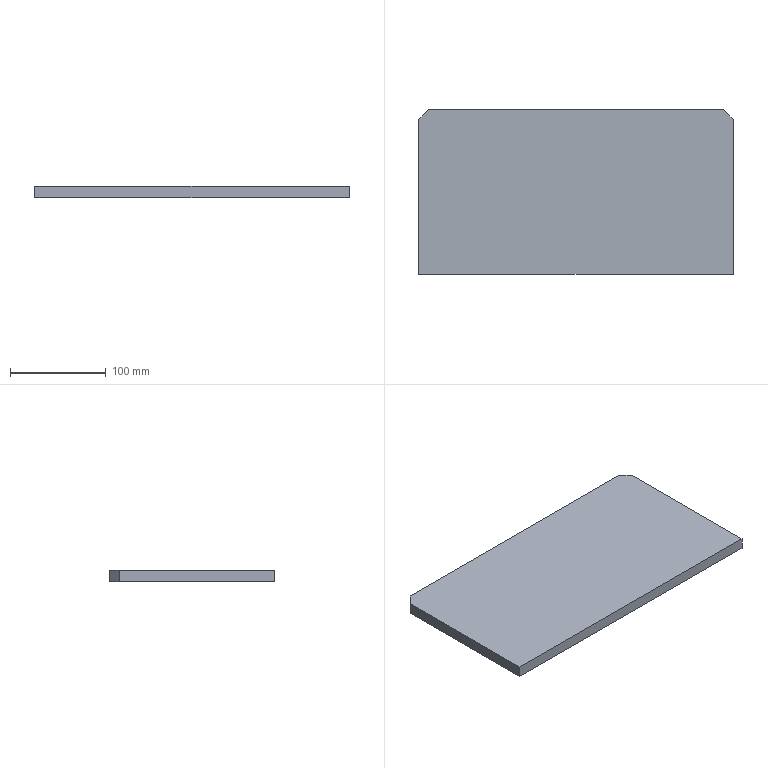Part | SolidWorks | features BaseBody 1 | 1 solid | 8 faces | box 328 x 172 x 12 mm | volume 675792 mm3 | plane 8
STEP:
#1=CARTESIAN_POINT('',(164.,-84.5,0.));
#2=VERTEX_POINT('',#1);
#3=CARTESIAN_POINT('',(164.,-84.5,12.));
#4=VERTEX_POINT('',#3);
#5=CARTESIAN_POINT('',(164.,-84.5,12.));
#6=DIRECTION('',(0.,0.,1.));
#7=VECTOR('',#6,1000.);
#8=LINE('',#5,#7);
#9=EDGE_CURVE('',#2,#4,#8,.T.);
#10=ORIENTED_EDGE('',*,*,#9,.F.);
#11=CARTESIAN_POINT('',(164.,77.5,0.));
#12=VERTEX_POINT('',#11);
#13=CARTESIAN_POINT('',(164.,77.5,0.));
#14=DIRECTION('',(0.,1.,0.));
#15=VECTOR('',#14,1000.);
#16=LINE('',#13,#15);
#17=EDGE_CURVE('',#2,#12,#16,.T.);
#18=ORIENTED_EDGE('',*,*,#17,.T.);
#19=CARTESIAN_POINT('',(164.,77.5,12.));
#20=VERTEX_POINT('',#19);
#21=CARTESIAN_POINT('',(164.,77.5,12.));
#22=DIRECTION('',(0.,0.,-1.));
#23=VECTOR('',#22,1000.);
#24=LINE('',#21,#23);
#25=EDGE_CURVE('',#20,#12,#24,.T.);
#26=ORIENTED_EDGE('',*,*,#25,.F.);
#27=CARTESIAN_POINT('',(164.,77.5,12.));
#28=DIRECTION('',(0.,1.,0.));
#29=VECTOR('',#28,1000.);
#30=LINE('',#27,#29);
#31=EDGE_CURVE('',#4,#20,#30,.T.);
#32=ORIENTED_EDGE('',*,*,#31,.F.);
#33=EDGE_LOOP('',(#10,#18,#26,#32));
#34=FACE_OUTER_BOUND('',#33,.T.);
#35=CARTESIAN_POINT('',(164.,77.5,12.));
#36=DIRECTION('',(-1.,0.,0.));
#37=DIRECTION('',(0.,0.,1.));
#38=AXIS2_PLACEMENT_3D('',#35,#36,#37);
#39=PLANE('',#38);
#40=ADVANCED_FACE('',(#34),#39,.F.);
#41=CARTESIAN_POINT('',(-164.,-84.5,12.));
#42=VERTEX_POINT('',#41);
#43=CARTESIAN_POINT('',(-164.,-84.5,0.));
#44=VERTEX_POINT('',#43);
#45=CARTESIAN_POINT('',(-164.,-84.5,12.));
#46=DIRECTION('',(0.,0.,-1.));
#47=VECTOR('',#46,1000.);
#48=LINE('',#45,#47);
#49=EDGE_CURVE('',#42,#44,#48,.T.);
#50=ORIENTED_EDGE('',*,*,#49,.F.);
#51=CARTESIAN_POINT('',(-164.,77.5,12.));
#52=VERTEX_POINT('',#51);
#53=CARTESIAN_POINT('',(-164.,77.5,12.));
#54=DIRECTION('',(0.,-1.,0.));
#55=VECTOR('',#54,1000.);
#56=LINE('',#53,#55);
#57=EDGE_CURVE('',#52,#42,#56,.T.);
#58=ORIENTED_EDGE('',*,*,#57,.F.);
#59=CARTESIAN_POINT('',(-164.,77.5,0.));
#60=VERTEX_POINT('',#59);
#61=CARTESIAN_POINT('',(-164.,77.5,12.));
#62=DIRECTION('',(0.,0.,-1.));
#63=VECTOR('',#62,1000.);
#64=LINE('',#61,#63);
#65=EDGE_CURVE('',#52,#60,#64,.T.);
#66=ORIENTED_EDGE('',*,*,#65,.T.);
#67=CARTESIAN_POINT('',(-164.,77.5,0.));
#68=DIRECTION('',(0.,-1.,0.));
#69=VECTOR('',#68,1000.);
#70=LINE('',#67,#69);
#71=EDGE_CURVE('',#60,#44,#70,.T.);
#72=ORIENTED_EDGE('',*,*,#71,.T.);
#73=EDGE_LOOP('',(#50,#58,#66,#72));
#74=FACE_OUTER_BOUND('',#73,.T.);
#75=CARTESIAN_POINT('',(-164.,77.5,12.));
#76=DIRECTION('',(1.,0.,0.));
#77=DIRECTION('',(0.,1.,0.));
#78=AXIS2_PLACEMENT_3D('',#75,#76,#77);
#79=PLANE('',#78);
#80=ADVANCED_FACE('',(#74),#79,.F.);
#81=ORIENTED_EDGE('',*,*,#57,.T.);
#82=CARTESIAN_POINT('',(0.,-84.5,12.));
#83=DIRECTION('',(1.,0.,0.));
#84=VECTOR('',#83,1000.);
#85=LINE('',#82,#84);
#86=EDGE_CURVE('',#42,#4,#85,.T.);
#87=ORIENTED_EDGE('',*,*,#86,.T.);
#88=ORIENTED_EDGE('',*,*,#31,.T.);
#89=CARTESIAN_POINT('',(154.,87.5,12.));
#90=VERTEX_POINT('',#89);
#91=CARTESIAN_POINT('',(154.,87.5,12.));
#92=DIRECTION('',(-0.7071,0.7071,0.));
#93=VECTOR('',#92,1000.);
#94=LINE('',#91,#93);
#95=EDGE_CURVE('',#20,#90,#94,.T.);
#96=ORIENTED_EDGE('',*,*,#95,.T.);
#97=CARTESIAN_POINT('',(-154.,87.5,12.));
#98=VERTEX_POINT('',#97);
#99=CARTESIAN_POINT('',(-154.,87.5,12.));
#100=DIRECTION('',(-1.,0.,0.));
#101=VECTOR('',#100,1000.);
#102=LINE('',#99,#101);
#103=EDGE_CURVE('',#90,#98,#102,.T.);
#104=ORIENTED_EDGE('',*,*,#103,.T.);
#105=CARTESIAN_POINT('',(-164.,77.5,12.));
#106=DIRECTION('',(-0.7071,-0.7071,0.));
#107=VECTOR('',#106,1000.);
#108=LINE('',#105,#107);
#109=EDGE_CURVE('',#98,#52,#108,.T.);
#110=ORIENTED_EDGE('',*,*,#109,.T.);
#111=EDGE_LOOP('',(#81,#87,#88,#96,#104,#110));
#112=FACE_OUTER_BOUND('',#111,.T.);
#113=CARTESIAN_POINT('',(0.,0.,12.));
#114=DIRECTION('',(0.,0.,1.));
#115=DIRECTION('',(1.,0.,0.));
#116=AXIS2_PLACEMENT_3D('',#113,#114,#115);
#117=PLANE('',#116);
#118=ADVANCED_FACE('',(#112),#117,.T.);
#119=CARTESIAN_POINT('',(0.,-84.5,0.));
#120=DIRECTION('',(1.,0.,0.));
#121=VECTOR('',#120,1000.);
#122=LINE('',#119,#121);
#123=EDGE_CURVE('',#44,#2,#122,.T.);
#124=ORIENTED_EDGE('',*,*,#123,.F.);
#125=ORIENTED_EDGE('',*,*,#71,.F.);
#126=CARTESIAN_POINT('',(-154.,87.5,0.));
#127=VERTEX_POINT('',#126);
#128=CARTESIAN_POINT('',(-164.,77.5,0.));
#129=DIRECTION('',(-0.7071,-0.7071,0.));
#130=VECTOR('',#129,1000.);
#131=LINE('',#128,#130);
#132=EDGE_CURVE('',#127,#60,#131,.T.);
#133=ORIENTED_EDGE('',*,*,#132,.F.);
#134=CARTESIAN_POINT('',(154.,87.5,0.));
#135=VERTEX_POINT('',#134);
#136=CARTESIAN_POINT('',(-154.,87.5,0.));
#137=DIRECTION('',(-1.,0.,0.));
#138=VECTOR('',#137,1000.);
#139=LINE('',#136,#138);
#140=EDGE_CURVE('',#135,#127,#139,.T.);
#141=ORIENTED_EDGE('',*,*,#140,.F.);
#142=CARTESIAN_POINT('',(154.,87.5,0.));
#143=DIRECTION('',(-0.7071,0.7071,0.));
#144=VECTOR('',#143,1000.);
#145=LINE('',#142,#144);
#146=EDGE_CURVE('',#12,#135,#145,.T.);
#147=ORIENTED_EDGE('',*,*,#146,.F.);
#148=ORIENTED_EDGE('',*,*,#17,.F.);
#149=EDGE_LOOP('',(#124,#125,#133,#141,#147,#148));
#150=FACE_OUTER_BOUND('',#149,.T.);
#151=CARTESIAN_POINT('',(0.,0.,0.));
#152=DIRECTION('',(0.,0.,1.));
#153=DIRECTION('',(1.,0.,0.));
#154=AXIS2_PLACEMENT_3D('',#151,#152,#153);
#155=PLANE('',#154);
#156=ADVANCED_FACE('',(#150),#155,.F.);
#157=ORIENTED_EDGE('',*,*,#146,.T.);
#158=CARTESIAN_POINT('',(154.,87.5,12.));
#159=DIRECTION('',(0.,0.,-1.));
#160=VECTOR('',#159,1000.);
#161=LINE('',#158,#160);
#162=EDGE_CURVE('',#90,#135,#161,.T.);
#163=ORIENTED_EDGE('',*,*,#162,.F.);
#164=ORIENTED_EDGE('',*,*,#95,.F.);
#165=ORIENTED_EDGE('',*,*,#25,.T.);
#166=EDGE_LOOP('',(#157,#163,#164,#165));
#167=FACE_OUTER_BOUND('',#166,.T.);
#168=CARTESIAN_POINT('',(154.,87.5,12.));
#169=DIRECTION('',(-0.7071,-0.7071,0.));
#170=DIRECTION('',(0.7071,-0.7071,0.));
#171=AXIS2_PLACEMENT_3D('',#168,#169,#170);
#172=PLANE('',#171);
#173=ADVANCED_FACE('',(#167),#172,.F.);
#174=ORIENTED_EDGE('',*,*,#140,.T.);
#175=CARTESIAN_POINT('',(-154.,87.5,12.));
#176=DIRECTION('',(0.,0.,-1.));
#177=VECTOR('',#176,1000.);
#178=LINE('',#175,#177);
#179=EDGE_CURVE('',#98,#127,#178,.T.);
#180=ORIENTED_EDGE('',*,*,#179,.F.);
#181=ORIENTED_EDGE('',*,*,#103,.F.);
#182=ORIENTED_EDGE('',*,*,#162,.T.);
#183=EDGE_LOOP('',(#174,#180,#181,#182));
#184=FACE_OUTER_BOUND('',#183,.T.);
#185=CARTESIAN_POINT('',(-154.,87.5,12.));
#186=DIRECTION('',(0.,-1.,0.));
#187=DIRECTION('',(0.,0.,-1.));
#188=AXIS2_PLACEMENT_3D('',#185,#186,#187);
#189=PLANE('',#188);
#190=ADVANCED_FACE('',(#184),#189,.F.);
#191=ORIENTED_EDGE('',*,*,#132,.T.);
#192=ORIENTED_EDGE('',*,*,#65,.F.);
#193=ORIENTED_EDGE('',*,*,#109,.F.);
#194=ORIENTED_EDGE('',*,*,#179,.T.);
#195=EDGE_LOOP('',(#191,#192,#193,#194));
#196=FACE_OUTER_BOUND('',#195,.T.);
#197=CARTESIAN_POINT('',(-164.,77.5,12.));
#198=DIRECTION('',(0.7071,-0.7071,0.));
#199=DIRECTION('',(0.7071,0.7071,0.));
#200=AXIS2_PLACEMENT_3D('',#197,#198,#199);
#201=PLANE('',#200);
#202=ADVANCED_FACE('',(#196),#201,.F.);
#203=ORIENTED_EDGE('',*,*,#49,.T.);
#204=ORIENTED_EDGE('',*,*,#123,.T.);
#205=ORIENTED_EDGE('',*,*,#9,.T.);
#206=ORIENTED_EDGE('',*,*,#86,.F.);
#207=EDGE_LOOP('',(#203,#204,#205,#206));
#208=FACE_OUTER_BOUND('',#207,.T.);
#209=CARTESIAN_POINT('',(170.,-84.5,6.));
#210=DIRECTION('',(0.,-1.,0.));
#211=DIRECTION('',(0.,0.,-1.));
#212=AXIS2_PLACEMENT_3D('',#209,#210,#211);
#213=PLANE('',#212);
#214=ADVANCED_FACE('',(#208),#213,.T.);
#215=CLOSED_SHELL('',(#40,#80,#118,#156,#173,#190,#202,#214));
#216=MANIFOLD_SOLID_BREP('',#215);
#217=CARTESIAN_POINT('',(0.,0.,0.));
#218=DIRECTION('',(0.,0.,1.));
#219=DIRECTION('',(1.,0.,0.));
#220=AXIS2_PLACEMENT_3D('',#217,#218,#219);
#221=(LENGTH_UNIT()NAMED_UNIT(*)SI_UNIT(.MILLI.,.METRE.));
#222=UNCERTAINTY_MEASURE_WITH_UNIT(LENGTH_MEASURE(0.00001),#221,'','');
#223=(NAMED_UNIT(*)PLANE_ANGLE_UNIT()SI_UNIT($,.RADIAN.));
#224=(NAMED_UNIT(*)SI_UNIT($,.STERADIAN.)SOLID_ANGLE_UNIT());
#225=(GEOMETRIC_REPRESENTATION_CONTEXT(3)GLOBAL_UNCERTAINTY_ASSIGNED_CONTEXT((#222))GLOBAL_UNIT_ASSIGNED_CONTEXT((#221,#223,#224))REPRESENTATION_CONTEXT('',''));
#226=ADVANCED_BREP_SHAPE_REPRESENTATION('',(#216,#220),#225);